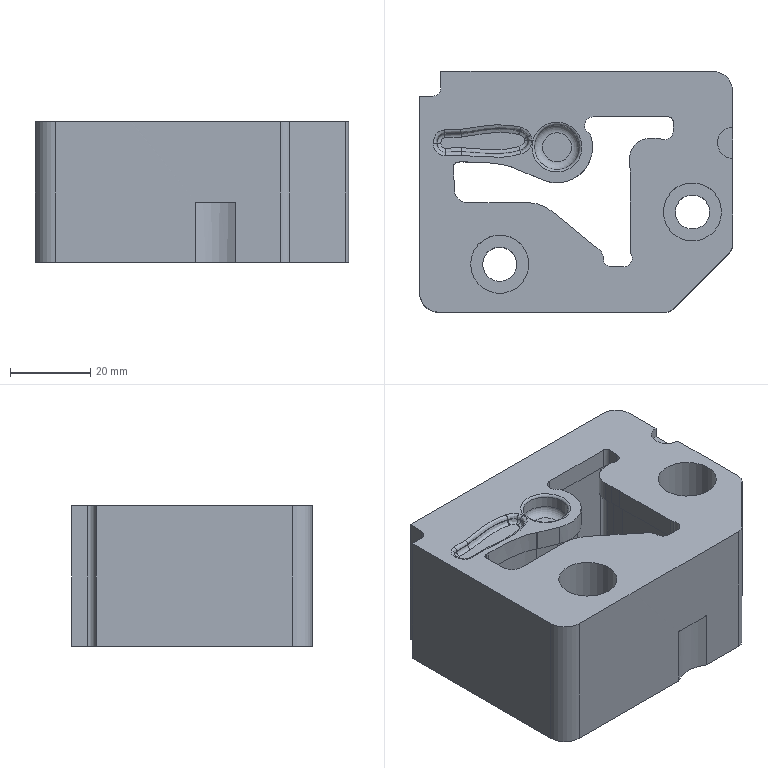Part | NX | features DIE-38 2 | 1 solid | 119 faces | box 78 x 60 x 35 mm | volume 119184 mm3 | spline 66 | plane 38 | cylinder 13 | torus 2 | commonest cylinder face diameters 6 x2 8.506 x2 10 x2 14.5 x2 1.8 x1 2 x1